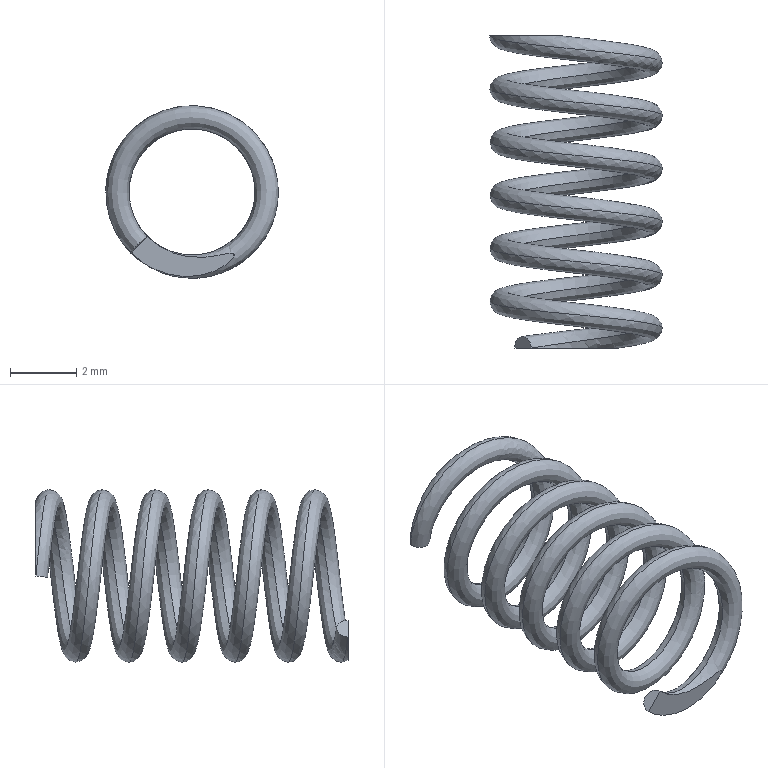Part | SolidWorks | features Helix 1, ICE 1, Sweep 1 | 1 solid | 6 faces | box 5.2 x 9.4 x 5.2 mm | volume 31.404 mm3 | plane 4 | spline 2